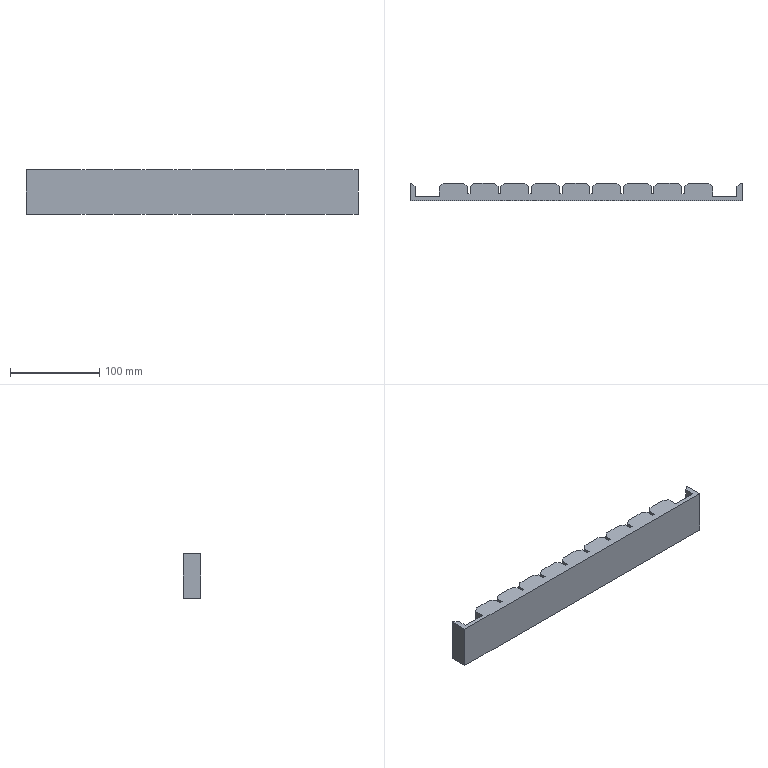Part | 1 solid | 66 faces | box 372.9 x 20 x 50 mm | volume 306700 mm3 | plane 66